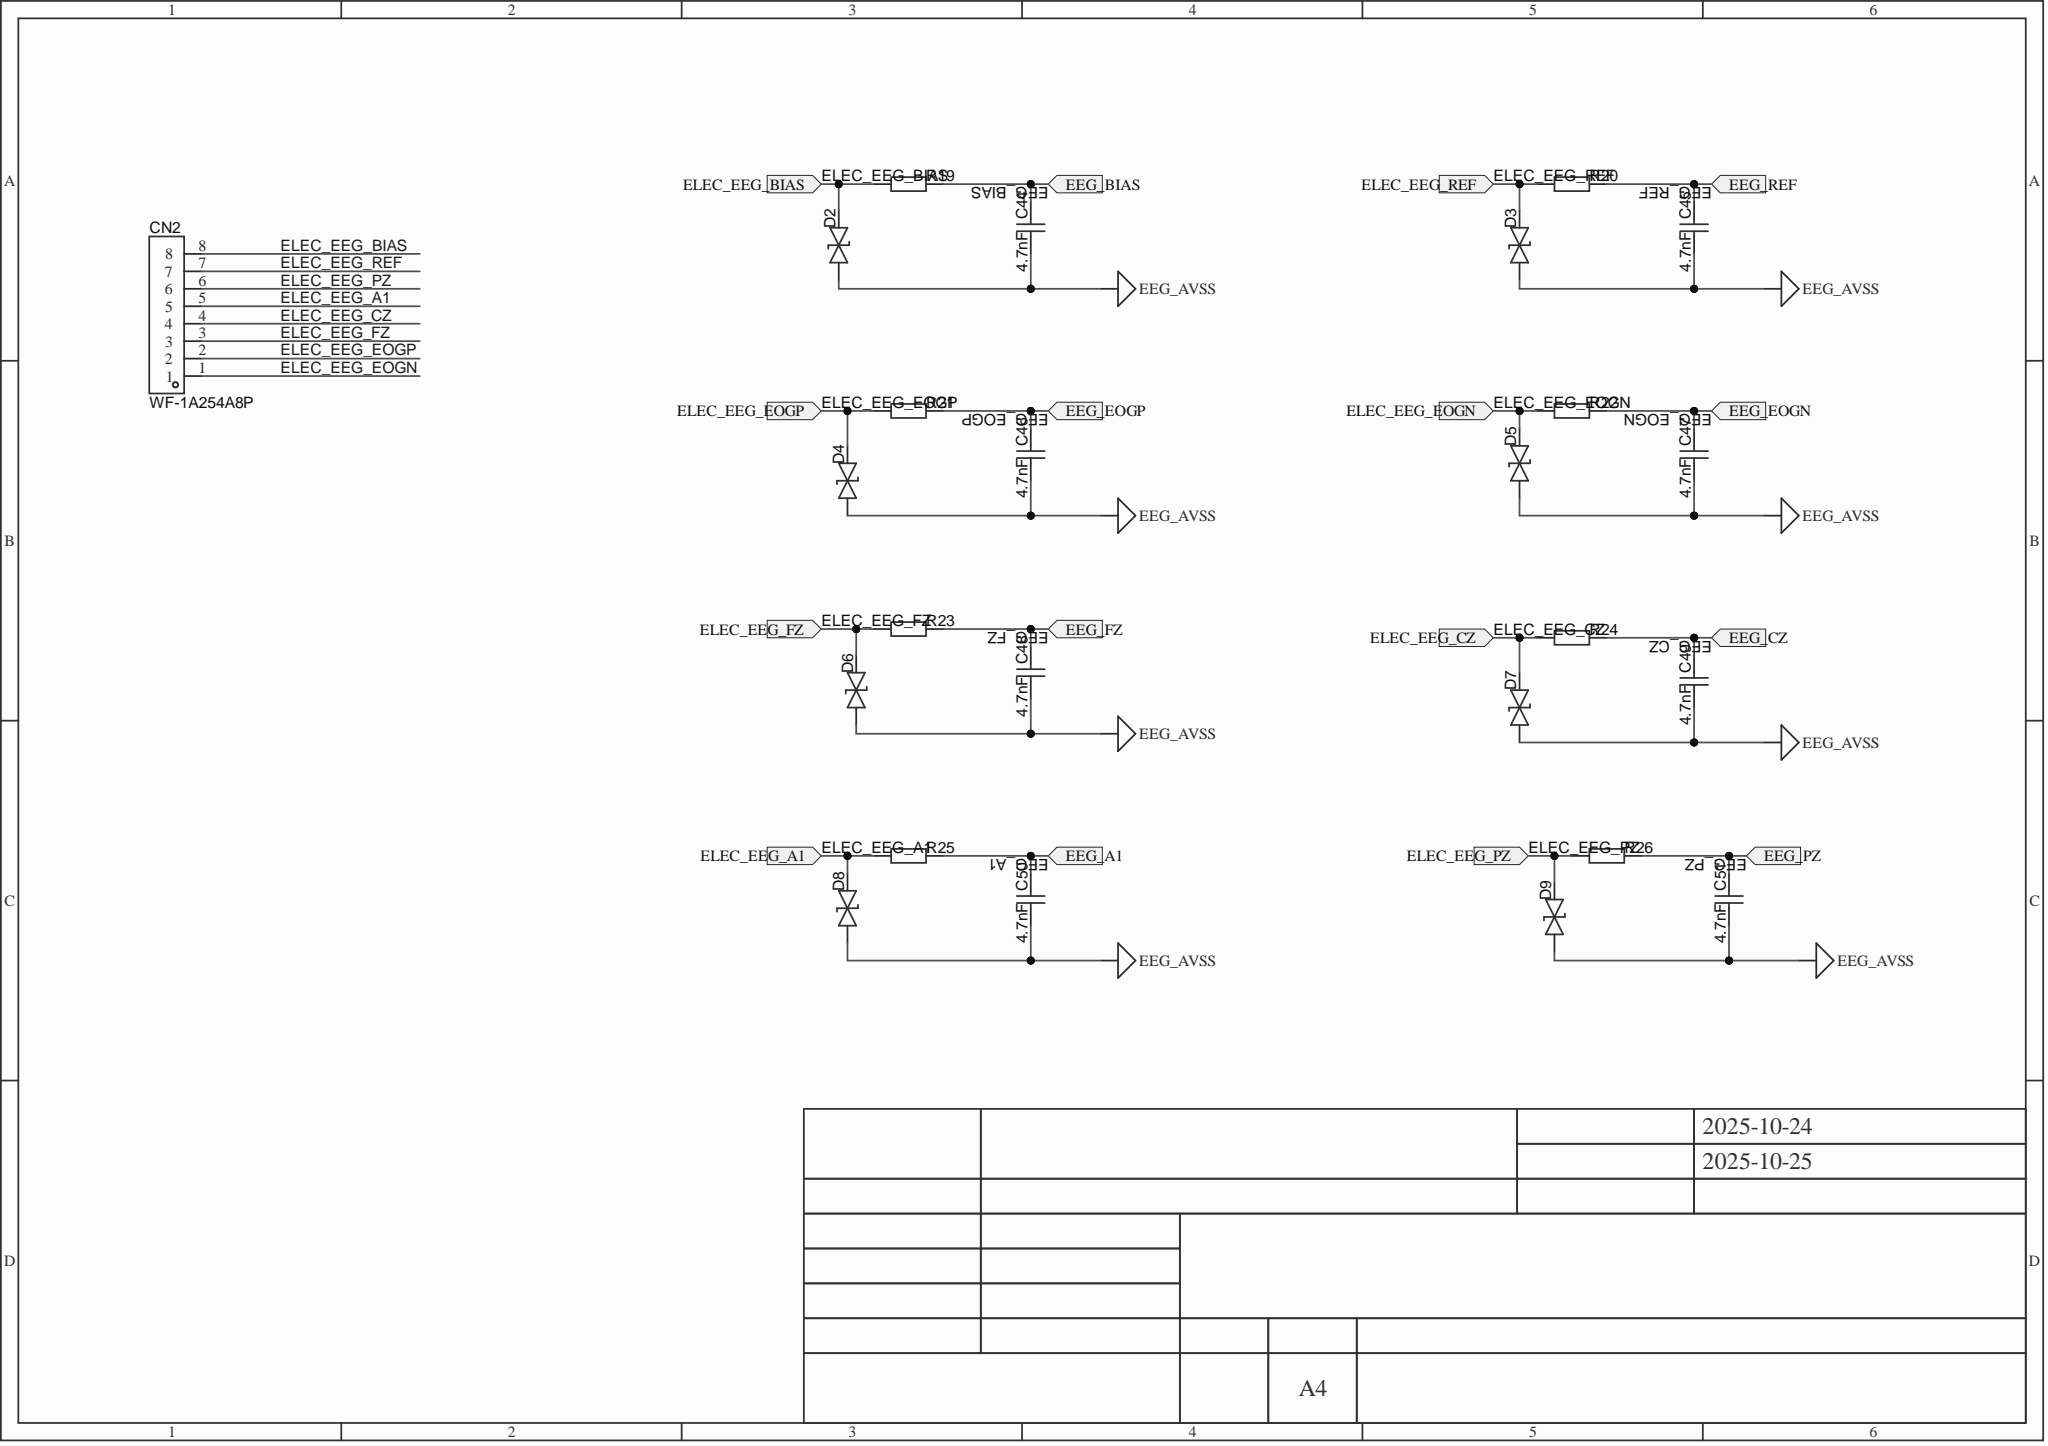Circuit board | Altium Designer | 211 parts | 126 nets | one sheet of the schematic
Parts on this sheet (reference | value | footprint):
C44 | 4.7nF | C0402
C45 | 4.7nF | C0402
C46 | 4.7nF | C0402
C47 | 4.7nF | C0402
C48 | 4.7nF | C0402
C49 | 4.7nF | C0402
C50 | 4.7nF | C0402
C51 | 4.7nF | C0402
CN2 | WF-1A254A8P | CONN-TH_WF-1A254A8P
D2 | TPD1E10B06DPYR-TP | X1-DFN1006-2_L1.0-W0.6-BI
D3 | TPD1E10B06DPYR-TP | X1-DFN1006-2_L1.0-W0.6-BI
D4 | TPD1E10B06DPYR-TP | X1-DFN1006-2_L1.0-W0.6-BI
D5 | TPD1E10B06DPYR-TP | X1-DFN1006-2_L1.0-W0.6-BI
D6 | TPD1E10B06DPYR-TP | X1-DFN1006-2_L1.0-W0.6-BI
D7 | TPD1E10B06DPYR-TP | X1-DFN1006-2_L1.0-W0.6-BI
D8 | TPD1E10B06DPYR-TP | X1-DFN1006-2_L1.0-W0.6-BI
D9 | TPD1E10B06DPYR-TP | X1-DFN1006-2_L1.0-W0.6-BI
R19 | R0402
R20 | R0402
R21 | R0402
R22 | R0402
R23 | R0402
R24 | R0402
R25 | R0402
R26 | R0402
Nets of these parts (net: part-pin ...):
ELEC_EEG_REF: CN2-7 D3-2 R20-1
ELEC_EEG_PZ: CN2-6 D9-2 R26-1
ELEC_EEG_FZ: CN2-3 D6-2 R23-1
ELEC_EEG_EOGP: CN2-2 D4-2 R21-1
ELEC_EEG_EOGN: CN2-1 D5-2 R22-1
ELEC_EEG_CZ: CN2-4 D7-2 R24-1
ELEC_EEG_BIAS: CN2-8 D2-2 R19-1
ELEC_EEG_A1: CN2-5 D8-2 R25-1
EEG_REF: C45-2 R20-2
EEG_PZ: C51-2 R26-2
EEG_FZ: C48-2 R23-2
EEG_EOGP: C46-2 R21-2
EEG_EOGN: C47-2 R22-2
EEG_CZ: C49-2 R24-2
EEG_BIAS: C44-2 R19-2
EEG_AVSS1: C44-1 C45-1 C46-1 C47-1 C48-1 C49-1 C50-1 C51-1 D2-1 D3-1 D4-1 D5-1 D6-1 D7-1 D8-1 D9-1
EEG_A1: C50-2 R25-2